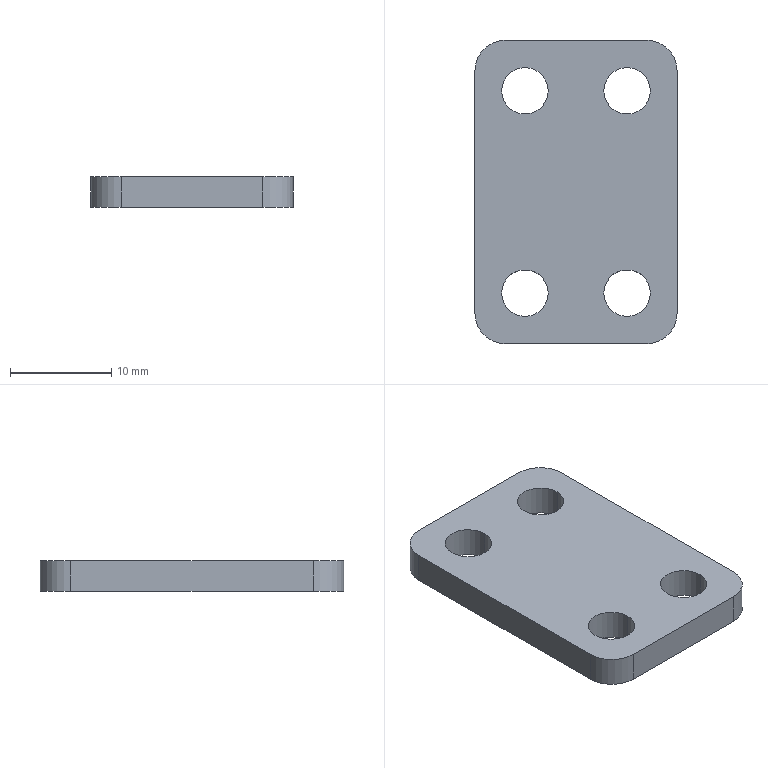Part | SolidWorks | features Extrusion 1, Fillet 1, ICE 1 | 1 solid | 18 faces | box 20 x 30 x 3 mm | volume 1577 mm3 | cylinder 12 | plane 6 | commonest cylinder face diameters 4.6 x8 6 x4
STEP:
#1=CARTESIAN_POINT('',(2.75,-10.,0.));
#2=VERTEX_POINT('',#1);
#3=CARTESIAN_POINT('',(7.35,-10.,0.));
#4=VERTEX_POINT('',#3);
#5=CARTESIAN_POINT('',(5.05,-10.,0.));
#6=DIRECTION('',(0.,0.,1.));
#7=DIRECTION('',(1.,0.,0.));
#8=AXIS2_PLACEMENT_3D('',#5,#6,#7);
#9=CIRCLE('',#8,2.3);
#10=EDGE_CURVE('',#2,#4,#9,.T.);
#11=ORIENTED_EDGE('',*,*,#10,.F.);
#12=CARTESIAN_POINT('',(2.75,-10.,3.));
#13=VERTEX_POINT('',#12);
#14=CARTESIAN_POINT('',(2.75,-10.,0.));
#15=DIRECTION('',(0.,0.,1.));
#16=VECTOR('',#15,1000.);
#17=LINE('',#14,#16);
#18=EDGE_CURVE('',#2,#13,#17,.T.);
#19=ORIENTED_EDGE('',*,*,#18,.T.);
#20=CARTESIAN_POINT('',(7.35,-10.,3.));
#21=VERTEX_POINT('',#20);
#22=CARTESIAN_POINT('',(5.05,-10.,3.));
#23=DIRECTION('',(0.,0.,1.));
#24=DIRECTION('',(1.,0.,0.));
#25=AXIS2_PLACEMENT_3D('',#22,#23,#24);
#26=CIRCLE('',#25,2.3);
#27=EDGE_CURVE('',#13,#21,#26,.T.);
#28=ORIENTED_EDGE('',*,*,#27,.T.);
#29=CARTESIAN_POINT('',(7.35,-10.,0.));
#30=DIRECTION('',(0.,0.,1.));
#31=VECTOR('',#30,1000.);
#32=LINE('',#29,#31);
#33=EDGE_CURVE('',#4,#21,#32,.T.);
#34=ORIENTED_EDGE('',*,*,#33,.F.);
#35=EDGE_LOOP('',(#11,#19,#28,#34));
#36=FACE_OUTER_BOUND('',#35,.T.);
#37=CARTESIAN_POINT('',(5.05,-10.,0.));
#38=DIRECTION('',(0.,0.,1.));
#39=DIRECTION('',(1.,0.,0.));
#40=AXIS2_PLACEMENT_3D('',#37,#38,#39);
#41=CYLINDRICAL_SURFACE('',#40,2.3);
#42=ADVANCED_FACE('',(#36),#41,.F.);
#43=CARTESIAN_POINT('',(-7.35,-10.,0.));
#44=VERTEX_POINT('',#43);
#45=CARTESIAN_POINT('',(-2.75,-10.,0.));
#46=VERTEX_POINT('',#45);
#47=CARTESIAN_POINT('',(-5.05,-10.,0.));
#48=DIRECTION('',(0.,0.,1.));
#49=DIRECTION('',(1.,0.,0.));
#50=AXIS2_PLACEMENT_3D('',#47,#48,#49);
#51=CIRCLE('',#50,2.3);
#52=EDGE_CURVE('',#44,#46,#51,.T.);
#53=ORIENTED_EDGE('',*,*,#52,.F.);
#54=CARTESIAN_POINT('',(-7.35,-10.,3.));
#55=VERTEX_POINT('',#54);
#56=CARTESIAN_POINT('',(-7.35,-10.,0.));
#57=DIRECTION('',(0.,0.,1.));
#58=VECTOR('',#57,1000.);
#59=LINE('',#56,#58);
#60=EDGE_CURVE('',#44,#55,#59,.T.);
#61=ORIENTED_EDGE('',*,*,#60,.T.);
#62=CARTESIAN_POINT('',(-2.75,-10.,3.));
#63=VERTEX_POINT('',#62);
#64=CARTESIAN_POINT('',(-5.05,-10.,3.));
#65=DIRECTION('',(0.,0.,1.));
#66=DIRECTION('',(1.,0.,0.));
#67=AXIS2_PLACEMENT_3D('',#64,#65,#66);
#68=CIRCLE('',#67,2.3);
#69=EDGE_CURVE('',#55,#63,#68,.T.);
#70=ORIENTED_EDGE('',*,*,#69,.T.);
#71=CARTESIAN_POINT('',(-2.75,-10.,0.));
#72=DIRECTION('',(0.,0.,1.));
#73=VECTOR('',#72,1000.);
#74=LINE('',#71,#73);
#75=EDGE_CURVE('',#46,#63,#74,.T.);
#76=ORIENTED_EDGE('',*,*,#75,.F.);
#77=EDGE_LOOP('',(#53,#61,#70,#76));
#78=FACE_OUTER_BOUND('',#77,.T.);
#79=CARTESIAN_POINT('',(-5.05,-10.,0.));
#80=DIRECTION('',(0.,0.,1.));
#81=DIRECTION('',(1.,0.,0.));
#82=AXIS2_PLACEMENT_3D('',#79,#80,#81);
#83=CYLINDRICAL_SURFACE('',#82,2.3);
#84=ADVANCED_FACE('',(#78),#83,.F.);
#85=CARTESIAN_POINT('',(2.75,10.,0.));
#86=VERTEX_POINT('',#85);
#87=CARTESIAN_POINT('',(7.35,10.,0.));
#88=VERTEX_POINT('',#87);
#89=CARTESIAN_POINT('',(5.05,10.,0.));
#90=DIRECTION('',(0.,0.,1.));
#91=DIRECTION('',(1.,0.,0.));
#92=AXIS2_PLACEMENT_3D('',#89,#90,#91);
#93=CIRCLE('',#92,2.3);
#94=EDGE_CURVE('',#86,#88,#93,.T.);
#95=ORIENTED_EDGE('',*,*,#94,.F.);
#96=CARTESIAN_POINT('',(2.75,10.,3.));
#97=VERTEX_POINT('',#96);
#98=CARTESIAN_POINT('',(2.75,10.,0.));
#99=DIRECTION('',(0.,0.,1.));
#100=VECTOR('',#99,1000.);
#101=LINE('',#98,#100);
#102=EDGE_CURVE('',#86,#97,#101,.T.);
#103=ORIENTED_EDGE('',*,*,#102,.T.);
#104=CARTESIAN_POINT('',(7.35,10.,3.));
#105=VERTEX_POINT('',#104);
#106=CARTESIAN_POINT('',(5.05,10.,3.));
#107=DIRECTION('',(0.,0.,1.));
#108=DIRECTION('',(1.,0.,0.));
#109=AXIS2_PLACEMENT_3D('',#106,#107,#108);
#110=CIRCLE('',#109,2.3);
#111=EDGE_CURVE('',#97,#105,#110,.T.);
#112=ORIENTED_EDGE('',*,*,#111,.T.);
#113=CARTESIAN_POINT('',(7.35,10.,0.));
#114=DIRECTION('',(0.,0.,1.));
#115=VECTOR('',#114,1000.);
#116=LINE('',#113,#115);
#117=EDGE_CURVE('',#88,#105,#116,.T.);
#118=ORIENTED_EDGE('',*,*,#117,.F.);
#119=EDGE_LOOP('',(#95,#103,#112,#118));
#120=FACE_OUTER_BOUND('',#119,.T.);
#121=CARTESIAN_POINT('',(5.05,10.,0.));
#122=DIRECTION('',(0.,0.,1.));
#123=DIRECTION('',(1.,0.,0.));
#124=AXIS2_PLACEMENT_3D('',#121,#122,#123);
#125=CYLINDRICAL_SURFACE('',#124,2.3);
#126=ADVANCED_FACE('',(#120),#125,.F.);
#127=CARTESIAN_POINT('',(-7.35,10.,0.));
#128=VERTEX_POINT('',#127);
#129=CARTESIAN_POINT('',(-2.75,10.,0.));
#130=VERTEX_POINT('',#129);
#131=CARTESIAN_POINT('',(-5.05,10.,0.));
#132=DIRECTION('',(0.,0.,1.));
#133=DIRECTION('',(1.,0.,0.));
#134=AXIS2_PLACEMENT_3D('',#131,#132,#133);
#135=CIRCLE('',#134,2.3);
#136=EDGE_CURVE('',#128,#130,#135,.T.);
#137=ORIENTED_EDGE('',*,*,#136,.F.);
#138=CARTESIAN_POINT('',(-7.35,10.,3.));
#139=VERTEX_POINT('',#138);
#140=CARTESIAN_POINT('',(-7.35,10.,0.));
#141=DIRECTION('',(0.,0.,1.));
#142=VECTOR('',#141,1000.);
#143=LINE('',#140,#142);
#144=EDGE_CURVE('',#128,#139,#143,.T.);
#145=ORIENTED_EDGE('',*,*,#144,.T.);
#146=CARTESIAN_POINT('',(-2.75,10.,3.));
#147=VERTEX_POINT('',#146);
#148=CARTESIAN_POINT('',(-5.05,10.,3.));
#149=DIRECTION('',(0.,0.,1.));
#150=DIRECTION('',(1.,0.,0.));
#151=AXIS2_PLACEMENT_3D('',#148,#149,#150);
#152=CIRCLE('',#151,2.3);
#153=EDGE_CURVE('',#139,#147,#152,.T.);
#154=ORIENTED_EDGE('',*,*,#153,.T.);
#155=CARTESIAN_POINT('',(-2.75,10.,0.));
#156=DIRECTION('',(0.,0.,1.));
#157=VECTOR('',#156,1000.);
#158=LINE('',#155,#157);
#159=EDGE_CURVE('',#130,#147,#158,.T.);
#160=ORIENTED_EDGE('',*,*,#159,.F.);
#161=EDGE_LOOP('',(#137,#145,#154,#160));
#162=FACE_OUTER_BOUND('',#161,.T.);
#163=CARTESIAN_POINT('',(-5.05,10.,0.));
#164=DIRECTION('',(0.,0.,1.));
#165=DIRECTION('',(1.,0.,0.));
#166=AXIS2_PLACEMENT_3D('',#163,#164,#165);
#167=CYLINDRICAL_SURFACE('',#166,2.3);
#168=ADVANCED_FACE('',(#162),#167,.F.);
#169=CARTESIAN_POINT('',(10.,-12.,3.));
#170=VERTEX_POINT('',#169);
#171=CARTESIAN_POINT('',(10.,12.,3.));
#172=VERTEX_POINT('',#171);
#173=CARTESIAN_POINT('',(10.,15.,3.));
#174=DIRECTION('',(0.,1.,0.));
#175=VECTOR('',#174,1000.);
#176=LINE('',#173,#175);
#177=EDGE_CURVE('',#170,#172,#176,.T.);
#178=ORIENTED_EDGE('',*,*,#177,.F.);
#179=CARTESIAN_POINT('',(10.,-12.,0.));
#180=VERTEX_POINT('',#179);
#181=CARTESIAN_POINT('',(10.,-12.,3.));
#182=DIRECTION('',(0.,0.,-1.));
#183=VECTOR('',#182,1000.);
#184=LINE('',#181,#183);
#185=EDGE_CURVE('',#170,#180,#184,.T.);
#186=ORIENTED_EDGE('',*,*,#185,.T.);
#187=CARTESIAN_POINT('',(10.,12.,0.));
#188=VERTEX_POINT('',#187);
#189=CARTESIAN_POINT('',(10.,15.,0.));
#190=DIRECTION('',(0.,1.,0.));
#191=VECTOR('',#190,1000.);
#192=LINE('',#189,#191);
#193=EDGE_CURVE('',#180,#188,#192,.T.);
#194=ORIENTED_EDGE('',*,*,#193,.T.);
#195=CARTESIAN_POINT('',(10.,12.,3.));
#196=DIRECTION('',(0.,0.,1.));
#197=VECTOR('',#196,1000.);
#198=LINE('',#195,#197);
#199=EDGE_CURVE('',#188,#172,#198,.T.);
#200=ORIENTED_EDGE('',*,*,#199,.T.);
#201=EDGE_LOOP('',(#178,#186,#194,#200));
#202=FACE_OUTER_BOUND('',#201,.T.);
#203=CARTESIAN_POINT('',(10.,15.,3.));
#204=DIRECTION('',(-1.,0.,0.));
#205=DIRECTION('',(0.,-1.,0.));
#206=AXIS2_PLACEMENT_3D('',#203,#204,#205);
#207=PLANE('',#206);
#208=ADVANCED_FACE('',(#202),#207,.F.);
#209=CARTESIAN_POINT('',(7.,15.,3.));
#210=VERTEX_POINT('',#209);
#211=CARTESIAN_POINT('',(-7.,15.,3.));
#212=VERTEX_POINT('',#211);
#213=CARTESIAN_POINT('',(-10.,15.,3.));
#214=DIRECTION('',(-1.,0.,0.));
#215=VECTOR('',#214,1000.);
#216=LINE('',#213,#215);
#217=EDGE_CURVE('',#210,#212,#216,.T.);
#218=ORIENTED_EDGE('',*,*,#217,.F.);
#219=CARTESIAN_POINT('',(7.,15.,0.));
#220=VERTEX_POINT('',#219);
#221=CARTESIAN_POINT('',(7.,15.,3.));
#222=DIRECTION('',(0.,0.,-1.));
#223=VECTOR('',#222,1000.);
#224=LINE('',#221,#223);
#225=EDGE_CURVE('',#210,#220,#224,.T.);
#226=ORIENTED_EDGE('',*,*,#225,.T.);
#227=CARTESIAN_POINT('',(-7.,15.,0.));
#228=VERTEX_POINT('',#227);
#229=CARTESIAN_POINT('',(-10.,15.,0.));
#230=DIRECTION('',(-1.,0.,0.));
#231=VECTOR('',#230,1000.);
#232=LINE('',#229,#231);
#233=EDGE_CURVE('',#220,#228,#232,.T.);
#234=ORIENTED_EDGE('',*,*,#233,.T.);
#235=CARTESIAN_POINT('',(-7.,15.,3.));
#236=DIRECTION('',(0.,0.,1.));
#237=VECTOR('',#236,1000.);
#238=LINE('',#235,#237);
#239=EDGE_CURVE('',#228,#212,#238,.T.);
#240=ORIENTED_EDGE('',*,*,#239,.T.);
#241=EDGE_LOOP('',(#218,#226,#234,#240));
#242=FACE_OUTER_BOUND('',#241,.T.);
#243=CARTESIAN_POINT('',(-10.,15.,3.));
#244=DIRECTION('',(0.,-1.,0.));
#245=DIRECTION('',(0.,0.,-1.));
#246=AXIS2_PLACEMENT_3D('',#243,#244,#245);
#247=PLANE('',#246);
#248=ADVANCED_FACE('',(#242),#247,.F.);
#249=CARTESIAN_POINT('',(-10.,12.,0.));
#250=VERTEX_POINT('',#249);
#251=CARTESIAN_POINT('',(-10.,-12.,0.));
#252=VERTEX_POINT('',#251);
#253=CARTESIAN_POINT('',(-10.,15.,0.));
#254=DIRECTION('',(0.,-1.,0.));
#255=VECTOR('',#254,1000.);
#256=LINE('',#253,#255);
#257=EDGE_CURVE('',#250,#252,#256,.T.);
#258=ORIENTED_EDGE('',*,*,#257,.T.);
#259=CARTESIAN_POINT('',(-10.,-12.,3.));
#260=VERTEX_POINT('',#259);
#261=CARTESIAN_POINT('',(-10.,-12.,3.));
#262=DIRECTION('',(0.,0.,1.));
#263=VECTOR('',#262,1000.);
#264=LINE('',#261,#263);
#265=EDGE_CURVE('',#252,#260,#264,.T.);
#266=ORIENTED_EDGE('',*,*,#265,.T.);
#267=CARTESIAN_POINT('',(-10.,12.,3.));
#268=VERTEX_POINT('',#267);
#269=CARTESIAN_POINT('',(-10.,15.,3.));
#270=DIRECTION('',(0.,-1.,0.));
#271=VECTOR('',#270,1000.);
#272=LINE('',#269,#271);
#273=EDGE_CURVE('',#268,#260,#272,.T.);
#274=ORIENTED_EDGE('',*,*,#273,.F.);
#275=CARTESIAN_POINT('',(-10.,12.,3.));
#276=DIRECTION('',(0.,0.,-1.));
#277=VECTOR('',#276,1000.);
#278=LINE('',#275,#277);
#279=EDGE_CURVE('',#268,#250,#278,.T.);
#280=ORIENTED_EDGE('',*,*,#279,.T.);
#281=EDGE_LOOP('',(#258,#266,#274,#280));
#282=FACE_OUTER_BOUND('',#281,.T.);
#283=CARTESIAN_POINT('',(-10.,15.,3.));
#284=DIRECTION('',(1.,0.,0.));
#285=DIRECTION('',(0.,1.,0.));
#286=AXIS2_PLACEMENT_3D('',#283,#284,#285);
#287=PLANE('',#286);
#288=ADVANCED_FACE('',(#282),#287,.F.);
#289=CARTESIAN_POINT('',(-7.,-15.,3.));
#290=VERTEX_POINT('',#289);
#291=CARTESIAN_POINT('',(7.,-15.,3.));
#292=VERTEX_POINT('',#291);
#293=CARTESIAN_POINT('',(-10.,-15.,3.));
#294=DIRECTION('',(1.,0.,0.));
#295=VECTOR('',#294,1000.);
#296=LINE('',#293,#295);
#297=EDGE_CURVE('',#290,#292,#296,.T.);
#298=ORIENTED_EDGE('',*,*,#297,.F.);
#299=CARTESIAN_POINT('',(-7.,-15.,0.));
#300=VERTEX_POINT('',#299);
#301=CARTESIAN_POINT('',(-7.,-15.,3.));
#302=DIRECTION('',(0.,0.,-1.));
#303=VECTOR('',#302,1000.);
#304=LINE('',#301,#303);
#305=EDGE_CURVE('',#290,#300,#304,.T.);
#306=ORIENTED_EDGE('',*,*,#305,.T.);
#307=CARTESIAN_POINT('',(7.,-15.,0.));
#308=VERTEX_POINT('',#307);
#309=CARTESIAN_POINT('',(-10.,-15.,0.));
#310=DIRECTION('',(1.,0.,0.));
#311=VECTOR('',#310,1000.);
#312=LINE('',#309,#311);
#313=EDGE_CURVE('',#300,#308,#312,.T.);
#314=ORIENTED_EDGE('',*,*,#313,.T.);
#315=CARTESIAN_POINT('',(7.,-15.,3.));
#316=DIRECTION('',(0.,0.,1.));
#317=VECTOR('',#316,1000.);
#318=LINE('',#315,#317);
#319=EDGE_CURVE('',#308,#292,#318,.T.);
#320=ORIENTED_EDGE('',*,*,#319,.T.);
#321=EDGE_LOOP('',(#298,#306,#314,#320));
#322=FACE_OUTER_BOUND('',#321,.T.);
#323=CARTESIAN_POINT('',(-10.,-15.,3.));
#324=DIRECTION('',(0.,1.,0.));
#325=DIRECTION('',(0.,0.,1.));
#326=AXIS2_PLACEMENT_3D('',#323,#324,#325);
#327=PLANE('',#326);
#328=ADVANCED_FACE('',(#322),#327,.F.);
#329=CARTESIAN_POINT('',(5.05,-10.,3.));
#330=DIRECTION('',(0.,0.,1.));
#331=DIRECTION('',(1.,0.,0.));
#332=AXIS2_PLACEMENT_3D('',#329,#330,#331);
#333=CIRCLE('',#332,2.3);
#334=EDGE_CURVE('',#21,#13,#333,.T.);
#335=ORIENTED_EDGE('',*,*,#334,.F.);
#336=ORIENTED_EDGE('',*,*,#27,.F.);
#337=EDGE_LOOP('',(#335,#336));
#338=FACE_BOUND('',#337,.T.);
#339=CARTESIAN_POINT('',(-5.05,-10.,3.));
#340=DIRECTION('',(0.,0.,1.));
#341=DIRECTION('',(1.,0.,0.));
#342=AXIS2_PLACEMENT_3D('',#339,#340,#341);
#343=CIRCLE('',#342,2.3);
#344=EDGE_CURVE('',#63,#55,#343,.T.);
#345=ORIENTED_EDGE('',*,*,#344,.F.);
#346=ORIENTED_EDGE('',*,*,#69,.F.);
#347=EDGE_LOOP('',(#345,#346));
#348=FACE_BOUND('',#347,.T.);
#349=CARTESIAN_POINT('',(5.05,10.,3.));
#350=DIRECTION('',(0.,0.,1.));
#351=DIRECTION('',(1.,0.,0.));
#352=AXIS2_PLACEMENT_3D('',#349,#350,#351);
#353=CIRCLE('',#352,2.3);
#354=EDGE_CURVE('',#105,#97,#353,.T.);
#355=ORIENTED_EDGE('',*,*,#354,.F.);
#356=ORIENTED_EDGE('',*,*,#111,.F.);
#357=EDGE_LOOP('',(#355,#356));
#358=FACE_BOUND('',#357,.T.);
#359=CARTESIAN_POINT('',(-5.05,10.,3.));
#360=DIRECTION('',(0.,0.,1.));
#361=DIRECTION('',(1.,0.,0.));
#362=AXIS2_PLACEMENT_3D('',#359,#360,#361);
#363=CIRCLE('',#362,2.3);
#364=EDGE_CURVE('',#147,#139,#363,.T.);
#365=ORIENTED_EDGE('',*,*,#364,.F.);
#366=ORIENTED_EDGE('',*,*,#153,.F.);
#367=EDGE_LOOP('',(#365,#366));
#368=FACE_BOUND('',#367,.T.);
#369=ORIENTED_EDGE('',*,*,#273,.T.);
#370=CARTESIAN_POINT('',(-7.,-12.,3.));
#371=DIRECTION('',(0.,0.,1.));
#372=DIRECTION('',(1.,0.,0.));
#373=AXIS2_PLACEMENT_3D('',#370,#371,#372);
#374=CIRCLE('',#373,3.);
#375=EDGE_CURVE('',#260,#290,#374,.T.);
#376=ORIENTED_EDGE('',*,*,#375,.T.);
#377=ORIENTED_EDGE('',*,*,#297,.T.);
#378=CARTESIAN_POINT('',(7.,-12.,3.));
#379=DIRECTION('',(0.,0.,1.));
#380=DIRECTION('',(1.,0.,0.));
#381=AXIS2_PLACEMENT_3D('',#378,#379,#380);
#382=CIRCLE('',#381,3.);
#383=EDGE_CURVE('',#292,#170,#382,.T.);
#384=ORIENTED_EDGE('',*,*,#383,.T.);
#385=ORIENTED_EDGE('',*,*,#177,.T.);
#386=CARTESIAN_POINT('',(7.,12.,3.));
#387=DIRECTION('',(0.,0.,1.));
#388=DIRECTION('',(1.,0.,0.));
#389=AXIS2_PLACEMENT_3D('',#386,#387,#388);
#390=CIRCLE('',#389,3.);
#391=EDGE_CURVE('',#172,#210,#390,.T.);
#392=ORIENTED_EDGE('',*,*,#391,.T.);
#393=ORIENTED_EDGE('',*,*,#217,.T.);
#394=CARTESIAN_POINT('',(-7.,12.,3.));
#395=DIRECTION('',(0.,0.,1.));
#396=DIRECTION('',(1.,0.,0.));
#397=AXIS2_PLACEMENT_3D('',#394,#395,#396);
#398=CIRCLE('',#397,3.);
#399=EDGE_CURVE('',#212,#268,#398,.T.);
#400=ORIENTED_EDGE('',*,*,#399,.T.);
#401=EDGE_LOOP('',(#369,#376,#377,#384,#385,#392,#393,#400));
#402=FACE_OUTER_BOUND('',#401,.T.);
#403=CARTESIAN_POINT('',(0.,0.,3.));
#404=DIRECTION('',(0.,0.,1.));
#405=DIRECTION('',(1.,0.,0.));
#406=AXIS2_PLACEMENT_3D('',#403,#404,#405);
#407=PLANE('',#406);
#408=ADVANCED_FACE('',(#338,#348,#358,#368,#402),#407,.T.);
#409=CARTESIAN_POINT('',(5.05,-10.,0.));
#410=DIRECTION('',(0.,0.,1.));
#411=DIRECTION('',(1.,0.,0.));
#412=AXIS2_PLACEMENT_3D('',#409,#410,#411);
#413=CIRCLE('',#412,2.3);
#414=EDGE_CURVE('',#4,#2,#413,.T.);
#415=ORIENTED_EDGE('',*,*,#414,.T.);
#416=ORIENTED_EDGE('',*,*,#10,.T.);
#417=EDGE_LOOP('',(#415,#416));
#418=FACE_BOUND('',#417,.T.);
#419=CARTESIAN_POINT('',(-5.05,-10.,0.));
#420=DIRECTION('',(0.,0.,1.));
#421=DIRECTION('',(1.,0.,0.));
#422=AXIS2_PLACEMENT_3D('',#419,#420,#421);
#423=CIRCLE('',#422,2.3);
#424=EDGE_CURVE('',#46,#44,#423,.T.);
#425=ORIENTED_EDGE('',*,*,#424,.T.);
#426=ORIENTED_EDGE('',*,*,#52,.T.);
#427=EDGE_LOOP('',(#425,#426));
#428=FACE_BOUND('',#427,.T.);
#429=CARTESIAN_POINT('',(5.05,10.,0.));
#430=DIRECTION('',(0.,0.,1.));
#431=DIRECTION('',(1.,0.,0.));
#432=AXIS2_PLACEMENT_3D('',#429,#430,#431);
#433=CIRCLE('',#432,2.3);
#434=EDGE_CURVE('',#88,#86,#433,.T.);
#435=ORIENTED_EDGE('',*,*,#434,.T.);
#436=ORIENTED_EDGE('',*,*,#94,.T.);
#437=EDGE_LOOP('',(#435,#436));
#438=FACE_BOUND('',#437,.T.);
#439=CARTESIAN_POINT('',(-5.05,10.,0.));
#440=DIRECTION('',(0.,0.,1.));
#441=DIRECTION('',(1.,0.,0.));
#442=AXIS2_PLACEMENT_3D('',#439,#440,#441);
#443=CIRCLE('',#442,2.3);
#444=EDGE_CURVE('',#130,#128,#443,.T.);
#445=ORIENTED_EDGE('',*,*,#444,.T.);
#446=ORIENTED_EDGE('',*,*,#136,.T.);
#447=EDGE_LOOP('',(#445,#446));
#448=FACE_BOUND('',#447,.T.);
#449=ORIENTED_EDGE('',*,*,#313,.F.);
#450=CARTESIAN_POINT('',(-7.,-12.,0.));
#451=DIRECTION('',(0.,0.,-1.));
#452=DIRECTION('',(1.,0.,0.));
#453=AXIS2_PLACEMENT_3D('',#450,#451,#452);
#454=CIRCLE('',#453,3.);
#455=EDGE_CURVE('',#300,#252,#454,.T.);
#456=ORIENTED_EDGE('',*,*,#455,.T.);
#457=ORIENTED_EDGE('',*,*,#257,.F.);
#458=CARTESIAN_POINT('',(-7.,12.,0.));
#459=DIRECTION('',(0.,0.,-1.));
#460=DIRECTION('',(1.,0.,0.));
#461=AXIS2_PLACEMENT_3D('',#458,#459,#460);
#462=CIRCLE('',#461,3.);
#463=EDGE_CURVE('',#250,#228,#462,.T.);
#464=ORIENTED_EDGE('',*,*,#463,.T.);
#465=ORIENTED_EDGE('',*,*,#233,.F.);
#466=CARTESIAN_POINT('',(7.,12.,0.));
#467=DIRECTION('',(0.,0.,-1.));
#468=DIRECTION('',(1.,0.,0.));
#469=AXIS2_PLACEMENT_3D('',#466,#467,#468);
#470=CIRCLE('',#469,3.);
#471=EDGE_CURVE('',#220,#188,#470,.T.);
#472=ORIENTED_EDGE('',*,*,#471,.T.);
#473=ORIENTED_EDGE('',*,*,#193,.F.);
#474=CARTESIAN_POINT('',(7.,-12.,0.));
#475=DIRECTION('',(0.,0.,-1.));
#476=DIRECTION('',(1.,0.,0.));
#477=AXIS2_PLACEMENT_3D('',#474,#475,#476);
#478=CIRCLE('',#477,3.);
#479=EDGE_CURVE('',#180,#308,#478,.T.);
#480=ORIENTED_EDGE('',*,*,#479,.T.);
#481=EDGE_LOOP('',(#449,#456,#457,#464,#465,#472,#473,#480));
#482=FACE_OUTER_BOUND('',#481,.T.);
#483=CARTESIAN_POINT('',(0.,0.,0.));
#484=DIRECTION('',(0.,0.,1.));
#485=DIRECTION('',(1.,0.,0.));
#486=AXIS2_PLACEMENT_3D('',#483,#484,#485);
#487=PLANE('',#486);
#488=ADVANCED_FACE('',(#418,#428,#438,#448,#482),#487,.F.);
#489=ORIENTED_EDGE('',*,*,#144,.F.);
#490=ORIENTED_EDGE('',*,*,#444,.F.);
#491=ORIENTED_EDGE('',*,*,#159,.T.);
#492=ORIENTED_EDGE('',*,*,#364,.T.);
#493=EDGE_LOOP('',(#489,#490,#491,#492));
#494=FACE_OUTER_BOUND('',#493,.T.);
#495=CARTESIAN_POINT('',(-5.05,10.,0.));
#496=DIRECTION('',(0.,0.,1.));
#497=DIRECTION('',(1.,0.,0.));
#498=AXIS2_PLACEMENT_3D('',#495,#496,#497);
#499=CYLINDRICAL_SURFACE('',#498,2.3);
#500=ADVANCED_FACE('',(#494),#499,.F.);
#501=ORIENTED_EDGE('',*,*,#102,.F.);
#502=ORIENTED_EDGE('',*,*,#434,.F.);
#503=ORIENTED_EDGE('',*,*,#117,.T.);
#504=ORIENTED_EDGE('',*,*,#354,.T.);
#505=EDGE_LOOP('',(#501,#502,#503,#504));
#506=FACE_OUTER_BOUND('',#505,.T.);
#507=CARTESIAN_POINT('',(5.05,10.,0.));
#508=DIRECTION('',(0.,0.,1.));
#509=DIRECTION('',(1.,0.,0.));
#510=AXIS2_PLACEMENT_3D('',#507,#508,#509);
#511=CYLINDRICAL_SURFACE('',#510,2.3);
#512=ADVANCED_FACE('',(#506),#511,.F.);
#513=ORIENTED_EDGE('',*,*,#60,.F.);
#514=ORIENTED_EDGE('',*,*,#424,.F.);
#515=ORIENTED_EDGE('',*,*,#75,.T.);
#516=ORIENTED_EDGE('',*,*,#344,.T.);
#517=EDGE_LOOP('',(#513,#514,#515,#516));
#518=FACE_OUTER_BOUND('',#517,.T.);
#519=CARTESIAN_POINT('',(-5.05,-10.,0.));
#520=DIRECTION('',(0.,0.,1.));
#521=DIRECTION('',(1.,0.,0.));
#522=AXIS2_PLACEMENT_3D('',#519,#520,#521);
#523=CYLINDRICAL_SURFACE('',#522,2.3);
#524=ADVANCED_FACE('',(#518),#523,.F.);
#525=ORIENTED_EDGE('',*,*,#18,.F.);
#526=ORIENTED_EDGE('',*,*,#414,.F.);
#527=ORIENTED_EDGE('',*,*,#33,.T.);
#528=ORIENTED_EDGE('',*,*,#334,.T.);
#529=EDGE_LOOP('',(#525,#526,#527,#528));
#530=FACE_OUTER_BOUND('',#529,.T.);
#531=CARTESIAN_POINT('',(5.05,-10.,0.));
#532=DIRECTION('',(0.,0.,1.));
#533=DIRECTION('',(1.,0.,0.));
#534=AXIS2_PLACEMENT_3D('',#531,#532,#533);
#535=CYLINDRICAL_SURFACE('',#534,2.3);
#536=ADVANCED_FACE('',(#530),#535,.F.);
#537=ORIENTED_EDGE('',*,*,#375,.F.);
#538=ORIENTED_EDGE('',*,*,#265,.F.);
#539=ORIENTED_EDGE('',*,*,#455,.F.);
#540=ORIENTED_EDGE('',*,*,#305,.F.);
#541=EDGE_LOOP('',(#537,#538,#539,#540));
#542=FACE_OUTER_BOUND('',#541,.T.);
#543=CARTESIAN_POINT('',(-7.,-12.,3.));
#544=DIRECTION('',(0.,0.,-1.));
#545=DIRECTION('',(-1.,0.,0.));
#546=AXIS2_PLACEMENT_3D('',#543,#544,#545);
#547=CYLINDRICAL_SURFACE('',#546,3.);
#548=ADVANCED_FACE('',(#542),#547,.T.);
#549=ORIENTED_EDGE('',*,*,#383,.F.);
#550=ORIENTED_EDGE('',*,*,#319,.F.);
#551=ORIENTED_EDGE('',*,*,#479,.F.);
#552=ORIENTED_EDGE('',*,*,#185,.F.);
#553=EDGE_LOOP('',(#549,#550,#551,#552));
#554=FACE_OUTER_BOUND('',#553,.T.);
#555=CARTESIAN_POINT('',(7.,-12.,3.));
#556=DIRECTION('',(0.,0.,-1.));
#557=DIRECTION('',(-1.,0.,0.));
#558=AXIS2_PLACEMENT_3D('',#555,#556,#557);
#559=CYLINDRICAL_SURFACE('',#558,3.);
#560=ADVANCED_FACE('',(#554),#559,.T.);
#561=ORIENTED_EDGE('',*,*,#391,.F.);
#562=ORIENTED_EDGE('',*,*,#199,.F.);
#563=ORIENTED_EDGE('',*,*,#471,.F.);
#564=ORIENTED_EDGE('',*,*,#225,.F.);
#565=EDGE_LOOP('',(#561,#562,#563,#564));
#566=FACE_OUTER_BOUND('',#565,.T.);
#567=CARTESIAN_POINT('',(7.,12.,3.));
#568=DIRECTION('',(0.,0.,-1.));
#569=DIRECTION('',(-1.,0.,0.));
#570=AXIS2_PLACEMENT_3D('',#567,#568,#569);
#571=CYLINDRICAL_SURFACE('',#570,3.);
#572=ADVANCED_FACE('',(#566),#571,.T.);
#573=ORIENTED_EDGE('',*,*,#399,.F.);
#574=ORIENTED_EDGE('',*,*,#239,.F.);
#575=ORIENTED_EDGE('',*,*,#463,.F.);
#576=ORIENTED_EDGE('',*,*,#279,.F.);
#577=EDGE_LOOP('',(#573,#574,#575,#576));
#578=FACE_OUTER_BOUND('',#577,.T.);
#579=CARTESIAN_POINT('',(-7.,12.,3.));
#580=DIRECTION('',(0.,0.,-1.));
#581=DIRECTION('',(-1.,0.,0.));
#582=AXIS2_PLACEMENT_3D('',#579,#580,#581);
#583=CYLINDRICAL_SURFACE('',#582,3.);
#584=ADVANCED_FACE('',(#578),#583,.T.);
#585=CLOSED_SHELL('',(#42,#84,#126,#168,#208,#248,#288,#328,#408,#488,#500,#512,#524,#536,#548,#560,#572,#584));
#586=MANIFOLD_SOLID_BREP('',#585);
#587=CARTESIAN_POINT('',(0.,0.,0.));
#588=DIRECTION('',(0.,0.,1.));
#589=DIRECTION('',(1.,0.,0.));
#590=AXIS2_PLACEMENT_3D('',#587,#588,#589);
#591=(LENGTH_UNIT()NAMED_UNIT(*)SI_UNIT(.MILLI.,.METRE.));
#592=UNCERTAINTY_MEASURE_WITH_UNIT(LENGTH_MEASURE(0.00001),#591,'','');
#593=(NAMED_UNIT(*)PLANE_ANGLE_UNIT()SI_UNIT($,.RADIAN.));
#594=(NAMED_UNIT(*)SI_UNIT($,.STERADIAN.)SOLID_ANGLE_UNIT());
#595=(GEOMETRIC_REPRESENTATION_CONTEXT(3)GLOBAL_UNCERTAINTY_ASSIGNED_CONTEXT((#592))GLOBAL_UNIT_ASSIGNED_CONTEXT((#591,#593,#594))REPRESENTATION_CONTEXT('',''));
#596=ADVANCED_BREP_SHAPE_REPRESENTATION('',(#586,#590),#595);